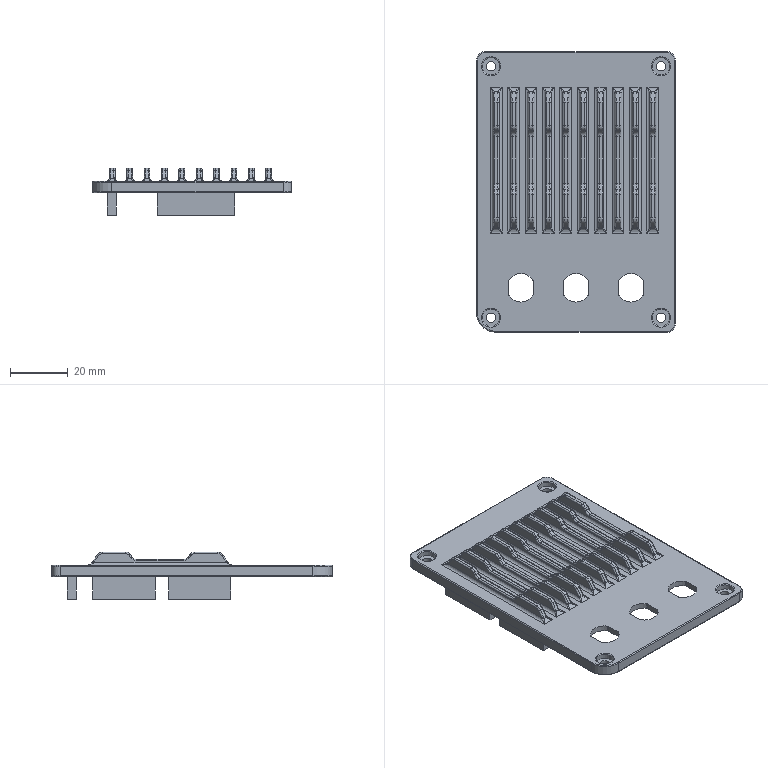Part | 1 solid | 658 faces | box 68.665 x 96.782 x 16.5 mm | volume 19561 mm3 | cylinder 294 | torus 144 | plane 140 | spline 80 | commonest cylinder face diameters 1 x140 4 x80 2 x32 0.6 x12 3.2 x12 9.9 x6